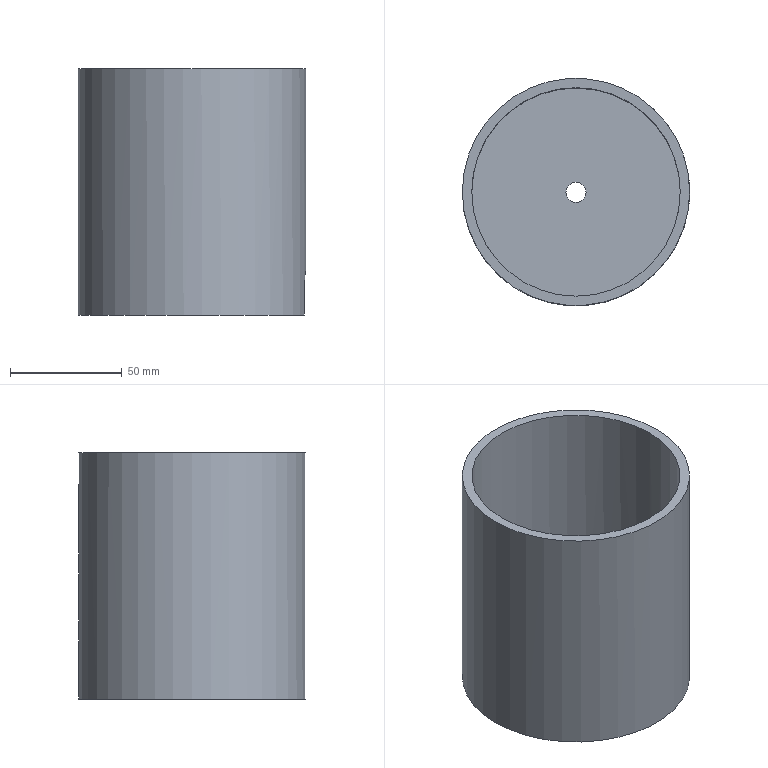Part | NX | features PHBTN70-140-110-Y_2 2 | 1 solid | 204 faces | box 101.6 x 101.6 x 110 mm | volume 150913 mm3 | plane 137 | cylinder 67 | commonest cylinder face diameters 101.4 x17 101.6 x8 3.09 x3 3.687 x3 3.698 x3 3.741 x3